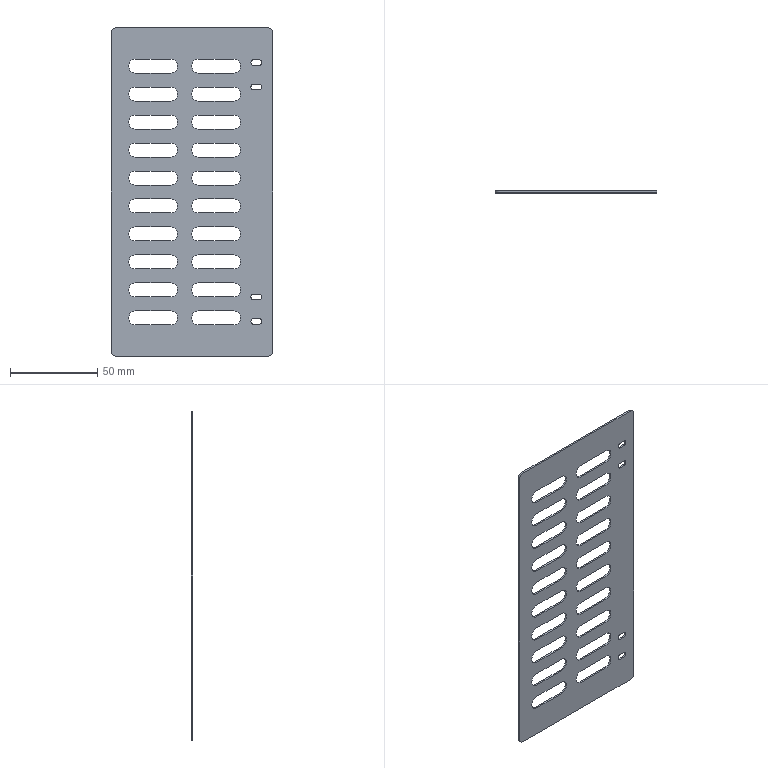Part | SolidWorks | features ICE 2, Extrusion 1, Fillet 1 | 1 solid | 106 faces | box 92.5 x 1 x 188 mm | volume 13106 mm3 | plane 54 | cylinder 52 | commonest cylinder face diameters 8 x40 3.2 x8 6 x4